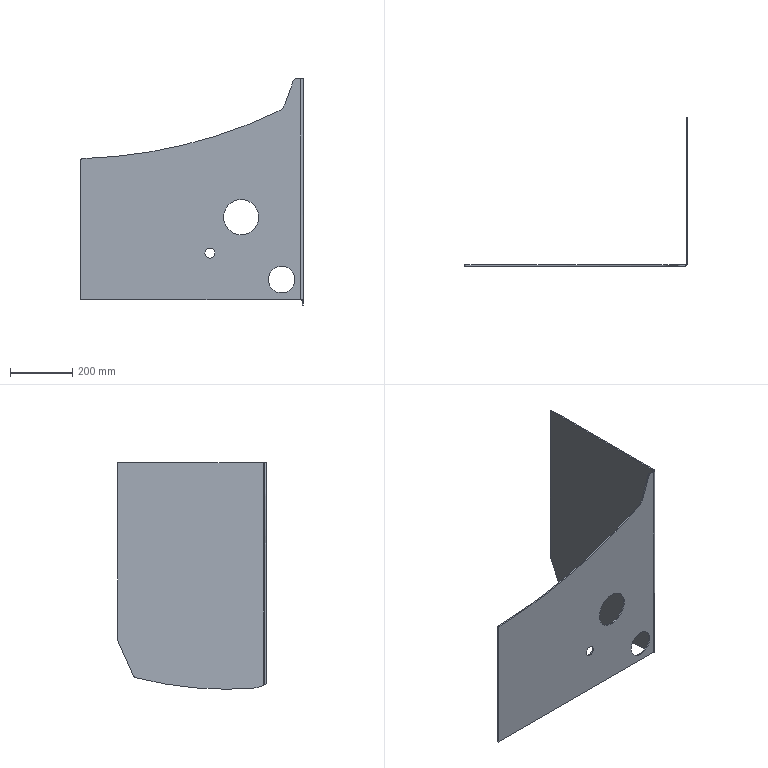Part | SolidWorks | features ICE 3, Fillet 2, FlatPattern 1, SMBaseFlange 1, SheetMetal 1 | 1 solid | 29 faces | box 715 x 476 x 726.29 mm | volume 2754090 mm3 | cylinder 15 | plane 13 | spline 1 | commonest cylinder face diameters 16 x3 20 x2 32.5 x2 85.5 x2 113 x2 12 x1
STEP:
#1=CARTESIAN_POINT('',(-283.75,-476.,-194.));
#2=VERTEX_POINT('',#1);
#3=CARTESIAN_POINT('',(-316.25,-476.,-194.));
#4=VERTEX_POINT('',#3);
#5=CARTESIAN_POINT('',(-300.,-476.,-194.));
#6=DIRECTION('',(0.,1.,0.));
#7=DIRECTION('',(1.,0.,0.));
#8=AXIS2_PLACEMENT_3D('',#5,#6,#7);
#9=CIRCLE('',#8,16.25);
#10=EDGE_CURVE('',#2,#4,#9,.T.);
#11=ORIENTED_EDGE('',*,*,#10,.F.);
#12=CARTESIAN_POINT('',(-283.75,-472.,-194.));
#13=VERTEX_POINT('',#12);
#14=CARTESIAN_POINT('',(-283.75,-476.001,-194.));
#15=DIRECTION('',(0.,1.,0.));
#16=VECTOR('',#15,1000.);
#17=LINE('',#14,#16);
#18=EDGE_CURVE('',#2,#13,#17,.T.);
#19=ORIENTED_EDGE('',*,*,#18,.T.);
#20=CARTESIAN_POINT('',(-316.25,-472.,-194.));
#21=VERTEX_POINT('',#20);
#22=CARTESIAN_POINT('',(-300.,-472.,-194.));
#23=DIRECTION('',(0.,1.,0.));
#24=DIRECTION('',(-1.,0.,0.));
#25=AXIS2_PLACEMENT_3D('',#22,#23,#24);
#26=CIRCLE('',#25,16.25);
#27=EDGE_CURVE('',#13,#21,#26,.T.);
#28=ORIENTED_EDGE('',*,*,#27,.T.);
#29=CARTESIAN_POINT('',(-316.25,-476.001,-194.));
#30=DIRECTION('',(0.,1.,0.));
#31=VECTOR('',#30,1000.);
#32=LINE('',#29,#31);
#33=EDGE_CURVE('',#4,#21,#32,.T.);
#34=ORIENTED_EDGE('',*,*,#33,.F.);
#35=EDGE_LOOP('',(#11,#19,#28,#34));
#36=FACE_OUTER_BOUND('',#35,.T.);
#37=CARTESIAN_POINT('',(-300.,-476.001,-194.));
#38=DIRECTION('',(0.,1.,0.));
#39=DIRECTION('',(-1.,0.,0.));
#40=AXIS2_PLACEMENT_3D('',#37,#38,#39);
#41=CYLINDRICAL_SURFACE('',#40,16.25);
#42=ADVANCED_FACE('',(#36),#41,.F.);
#43=CARTESIAN_POINT('',(-143.5,-476.,-79.));
#44=VERTEX_POINT('',#43);
#45=CARTESIAN_POINT('',(-256.5,-476.,-79.));
#46=VERTEX_POINT('',#45);
#47=CARTESIAN_POINT('',(-200.,-476.,-79.));
#48=DIRECTION('',(0.,1.,0.));
#49=DIRECTION('',(1.,0.,0.));
#50=AXIS2_PLACEMENT_3D('',#47,#48,#49);
#51=CIRCLE('',#50,56.5);
#52=EDGE_CURVE('',#44,#46,#51,.T.);
#53=ORIENTED_EDGE('',*,*,#52,.F.);
#54=CARTESIAN_POINT('',(-143.5,-472.,-79.));
#55=VERTEX_POINT('',#54);
#56=CARTESIAN_POINT('',(-143.5,-476.001,-79.));
#57=DIRECTION('',(0.,1.,0.));
#58=VECTOR('',#57,1000.);
#59=LINE('',#56,#58);
#60=EDGE_CURVE('',#44,#55,#59,.T.);
#61=ORIENTED_EDGE('',*,*,#60,.T.);
#62=CARTESIAN_POINT('',(-256.5,-472.,-79.));
#63=VERTEX_POINT('',#62);
#64=CARTESIAN_POINT('',(-200.,-472.,-79.));
#65=DIRECTION('',(0.,1.,0.));
#66=DIRECTION('',(-1.,0.,0.));
#67=AXIS2_PLACEMENT_3D('',#64,#65,#66);
#68=CIRCLE('',#67,56.5);
#69=EDGE_CURVE('',#55,#63,#68,.T.);
#70=ORIENTED_EDGE('',*,*,#69,.T.);
#71=CARTESIAN_POINT('',(-256.5,-476.001,-79.));
#72=DIRECTION('',(0.,1.,0.));
#73=VECTOR('',#72,1000.);
#74=LINE('',#71,#73);
#75=EDGE_CURVE('',#46,#63,#74,.T.);
#76=ORIENTED_EDGE('',*,*,#75,.F.);
#77=EDGE_LOOP('',(#53,#61,#70,#76));
#78=FACE_OUTER_BOUND('',#77,.T.);
#79=CARTESIAN_POINT('',(-200.,-476.001,-79.));
#80=DIRECTION('',(0.,1.,0.));
#81=DIRECTION('',(-1.,0.,0.));
#82=AXIS2_PLACEMENT_3D('',#79,#80,#81);
#83=CYLINDRICAL_SURFACE('',#82,56.5);
#84=ADVANCED_FACE('',(#78),#83,.F.);
#85=CARTESIAN_POINT('',(-27.25,-476.,-279.));
#86=VERTEX_POINT('',#85);
#87=CARTESIAN_POINT('',(-112.75,-476.,-279.));
#88=VERTEX_POINT('',#87);
#89=CARTESIAN_POINT('',(-70.,-476.,-279.));
#90=DIRECTION('',(0.,1.,0.));
#91=DIRECTION('',(1.,0.,0.));
#92=AXIS2_PLACEMENT_3D('',#89,#90,#91);
#93=CIRCLE('',#92,42.75);
#94=EDGE_CURVE('',#86,#88,#93,.T.);
#95=ORIENTED_EDGE('',*,*,#94,.F.);
#96=CARTESIAN_POINT('',(-27.25,-472.,-279.));
#97=VERTEX_POINT('',#96);
#98=CARTESIAN_POINT('',(-27.25,-476.001,-279.));
#99=DIRECTION('',(0.,1.,0.));
#100=VECTOR('',#99,1000.);
#101=LINE('',#98,#100);
#102=EDGE_CURVE('',#86,#97,#101,.T.);
#103=ORIENTED_EDGE('',*,*,#102,.T.);
#104=CARTESIAN_POINT('',(-112.75,-472.,-279.));
#105=VERTEX_POINT('',#104);
#106=CARTESIAN_POINT('',(-70.,-472.,-279.));
#107=DIRECTION('',(0.,1.,0.));
#108=DIRECTION('',(-1.,0.,0.));
#109=AXIS2_PLACEMENT_3D('',#106,#107,#108);
#110=CIRCLE('',#109,42.75);
#111=EDGE_CURVE('',#97,#105,#110,.T.);
#112=ORIENTED_EDGE('',*,*,#111,.T.);
#113=CARTESIAN_POINT('',(-112.75,-476.001,-279.));
#114=DIRECTION('',(0.,1.,0.));
#115=VECTOR('',#114,1000.);
#116=LINE('',#113,#115);
#117=EDGE_CURVE('',#88,#105,#116,.T.);
#118=ORIENTED_EDGE('',*,*,#117,.F.);
#119=EDGE_LOOP('',(#95,#103,#112,#118));
#120=FACE_OUTER_BOUND('',#119,.T.);
#121=CARTESIAN_POINT('',(-70.,-476.001,-279.));
#122=DIRECTION('',(0.,1.,0.));
#123=DIRECTION('',(-1.,0.,0.));
#124=AXIS2_PLACEMENT_3D('',#121,#122,#123);
#125=CYLINDRICAL_SURFACE('',#124,42.75);
#126=ADVANCED_FACE('',(#120),#125,.F.);
#127=CARTESIAN_POINT('',(-715.,-476.,101.209));
#128=VERTEX_POINT('',#127);
#129=CARTESIAN_POINT('',(-715.,-476.,-343.5));
#130=VERTEX_POINT('',#129);
#131=CARTESIAN_POINT('',(-715.,-476.,365.));
#132=DIRECTION('',(0.,0.,-1.));
#133=VECTOR('',#132,1000.);
#134=LINE('',#131,#133);
#135=EDGE_CURVE('',#128,#130,#134,.T.);
#136=ORIENTED_EDGE('',*,*,#135,.F.);
#137=CARTESIAN_POINT('',(-715.,-472.,101.209));
#138=VERTEX_POINT('',#137);
#139=CARTESIAN_POINT('',(-715.,-476.,101.209));
#140=DIRECTION('',(0.,1.,0.));
#141=VECTOR('',#140,1000.);
#142=LINE('',#139,#141);
#143=EDGE_CURVE('',#128,#138,#142,.T.);
#144=ORIENTED_EDGE('',*,*,#143,.T.);
#145=CARTESIAN_POINT('',(-715.,-472.,-343.5));
#146=VERTEX_POINT('',#145);
#147=CARTESIAN_POINT('',(-715.,-472.,365.));
#148=DIRECTION('',(0.,0.,-1.));
#149=VECTOR('',#148,1000.);
#150=LINE('',#147,#149);
#151=EDGE_CURVE('',#138,#146,#150,.T.);
#152=ORIENTED_EDGE('',*,*,#151,.T.);
#153=CARTESIAN_POINT('',(-715.,-476.,-343.5));
#154=DIRECTION('',(0.,1.,0.));
#155=VECTOR('',#154,1000.);
#156=LINE('',#153,#155);
#157=EDGE_CURVE('',#130,#146,#156,.T.);
#158=ORIENTED_EDGE('',*,*,#157,.F.);
#159=EDGE_LOOP('',(#136,#144,#152,#158));
#160=FACE_OUTER_BOUND('',#159,.T.);
#161=CARTESIAN_POINT('',(-715.,-476.,365.));
#162=DIRECTION('',(-1.,0.,0.));
#163=DIRECTION('',(0.,0.,1.));
#164=AXIS2_PLACEMENT_3D('',#161,#162,#163);
#165=PLANE('',#164);
#166=ADVANCED_FACE('',(#160),#165,.T.);
#167=CARTESIAN_POINT('',(-300.,-472.,-194.));
#168=DIRECTION('',(0.,1.,0.));
#169=DIRECTION('',(-1.,0.,0.));
#170=AXIS2_PLACEMENT_3D('',#167,#168,#169);
#171=CIRCLE('',#170,16.25);
#172=EDGE_CURVE('',#21,#13,#171,.T.);
#173=ORIENTED_EDGE('',*,*,#172,.F.);
#174=ORIENTED_EDGE('',*,*,#27,.F.);
#175=EDGE_LOOP('',(#173,#174));
#176=FACE_BOUND('',#175,.T.);
#177=CARTESIAN_POINT('',(-200.,-472.,-79.));
#178=DIRECTION('',(0.,1.,0.));
#179=DIRECTION('',(-1.,0.,0.));
#180=AXIS2_PLACEMENT_3D('',#177,#178,#179);
#181=CIRCLE('',#180,56.5);
#182=EDGE_CURVE('',#63,#55,#181,.T.);
#183=ORIENTED_EDGE('',*,*,#182,.F.);
#184=ORIENTED_EDGE('',*,*,#69,.F.);
#185=EDGE_LOOP('',(#183,#184));
#186=FACE_BOUND('',#185,.T.);
#187=CARTESIAN_POINT('',(-70.,-472.,-279.));
#188=DIRECTION('',(0.,1.,0.));
#189=DIRECTION('',(-1.,0.,0.));
#190=AXIS2_PLACEMENT_3D('',#187,#188,#189);
#191=CIRCLE('',#190,42.75);
#192=EDGE_CURVE('',#105,#97,#191,.T.);
#193=ORIENTED_EDGE('',*,*,#192,.F.);
#194=ORIENTED_EDGE('',*,*,#111,.F.);
#195=EDGE_LOOP('',(#193,#194));
#196=FACE_BOUND('',#195,.T.);
#197=ORIENTED_EDGE('',*,*,#151,.F.);
#198=CARTESIAN_POINT('',(-707.231,-472.,109.205));
#199=VERTEX_POINT('',#198);
#200=CARTESIAN_POINT('',(-707.,-472.,101.209));
#201=DIRECTION('',(0.,1.,0.));
#202=DIRECTION('',(1.,0.,0.));
#203=AXIS2_PLACEMENT_3D('',#200,#201,#202);
#204=CIRCLE('',#203,8.);
#205=EDGE_CURVE('',#138,#199,#204,.T.);
#206=ORIENTED_EDGE('',*,*,#205,.T.);
#207=CARTESIAN_POINT('',(-82.003,-472.,259.931));
#208=VERTEX_POINT('',#207);
#209=CARTESIAN_POINT('',(-752.366,-472.,1668.552));
#210=DIRECTION('',(0.,1.,0.));
#211=DIRECTION('',(1.,0.,0.));
#212=AXIS2_PLACEMENT_3D('',#209,#210,#211);
#213=CIRCLE('',#212,1560.);
#214=EDGE_CURVE('',#208,#199,#213,.T.);
#215=ORIENTED_EDGE('',*,*,#214,.F.);
#216=CARTESIAN_POINT('',(-59.054,-472.,285.174));
#217=VERTEX_POINT('',#216);
#218=CARTESIAN_POINT('',(-101.341,-472.,300.565));
#219=DIRECTION('',(0.,1.,0.));
#220=DIRECTION('',(1.,0.,0.));
#221=AXIS2_PLACEMENT_3D('',#218,#219,#220);
#222=CIRCLE('',#221,45.);
#223=EDGE_CURVE('',#217,#208,#222,.T.);
#224=ORIENTED_EDGE('',*,*,#223,.F.);
#225=CARTESIAN_POINT('',(-32.395,-472.,358.42));
#226=VERTEX_POINT('',#225);
#227=CARTESIAN_POINT('',(-30.,-472.,365.));
#228=DIRECTION('',(-0.342,0.,-0.9397));
#229=VECTOR('',#228,1000.);
#230=LINE('',#227,#229);
#231=EDGE_CURVE('',#226,#217,#230,.T.);
#232=ORIENTED_EDGE('',*,*,#231,.F.);
#233=CARTESIAN_POINT('',(-22.998,-472.,365.));
#234=VERTEX_POINT('',#233);
#235=CARTESIAN_POINT('',(-22.998,-472.,355.));
#236=DIRECTION('',(0.,1.,0.));
#237=DIRECTION('',(1.,0.,0.));
#238=AXIS2_PLACEMENT_3D('',#235,#236,#237);
#239=CIRCLE('',#238,10.);
#240=EDGE_CURVE('',#226,#234,#239,.T.);
#241=ORIENTED_EDGE('',*,*,#240,.T.);
#242=CARTESIAN_POINT('',(-10.,-472.,365.));
#243=VERTEX_POINT('',#242);
#244=CARTESIAN_POINT('',(0.,-472.,365.));
#245=DIRECTION('',(-1.,0.,0.));
#246=VECTOR('',#245,1000.);
#247=LINE('',#244,#246);
#248=EDGE_CURVE('',#243,#234,#247,.T.);
#249=ORIENTED_EDGE('',*,*,#248,.F.);
#250=CARTESIAN_POINT('',(-10.,-472.,-343.5));
#251=VERTEX_POINT('',#250);
#252=CARTESIAN_POINT('',(-10.,-472.,365.));
#253=DIRECTION('',(0.,0.,-1.));
#254=VECTOR('',#253,1000.);
#255=LINE('',#252,#254);
#256=EDGE_CURVE('',#243,#251,#255,.T.);
#257=ORIENTED_EDGE('',*,*,#256,.T.);
#258=CARTESIAN_POINT('',(0.,-472.,-343.5));
#259=DIRECTION('',(-1.,0.,0.));
#260=VECTOR('',#259,1000.);
#261=LINE('',#258,#260);
#262=EDGE_CURVE('',#251,#146,#261,.T.);
#263=ORIENTED_EDGE('',*,*,#262,.T.);
#264=EDGE_LOOP('',(#197,#206,#215,#224,#232,#241,#249,#257,#263));
#265=FACE_OUTER_BOUND('',#264,.T.);
#266=CARTESIAN_POINT('',(0.,-472.,365.));
#267=DIRECTION('',(0.,-1.,0.));
#268=DIRECTION('',(1.,0.,0.));
#269=AXIS2_PLACEMENT_3D('',#266,#267,#268);
#270=PLANE('',#269);
#271=ADVANCED_FACE('',(#176,#186,#196,#265),#270,.F.);
#272=CARTESIAN_POINT('',(-300.,-476.,-194.));
#273=DIRECTION('',(0.,1.,0.));
#274=DIRECTION('',(1.,0.,0.));
#275=AXIS2_PLACEMENT_3D('',#272,#273,#274);
#276=CIRCLE('',#275,16.25);
#277=EDGE_CURVE('',#4,#2,#276,.T.);
#278=ORIENTED_EDGE('',*,*,#277,.T.);
#279=ORIENTED_EDGE('',*,*,#10,.T.);
#280=EDGE_LOOP('',(#278,#279));
#281=FACE_BOUND('',#280,.T.);
#282=CARTESIAN_POINT('',(-200.,-476.,-79.));
#283=DIRECTION('',(0.,1.,0.));
#284=DIRECTION('',(1.,0.,0.));
#285=AXIS2_PLACEMENT_3D('',#282,#283,#284);
#286=CIRCLE('',#285,56.5);
#287=EDGE_CURVE('',#46,#44,#286,.T.);
#288=ORIENTED_EDGE('',*,*,#287,.T.);
#289=ORIENTED_EDGE('',*,*,#52,.T.);
#290=EDGE_LOOP('',(#288,#289));
#291=FACE_BOUND('',#290,.T.);
#292=CARTESIAN_POINT('',(-70.,-476.,-279.));
#293=DIRECTION('',(0.,1.,0.));
#294=DIRECTION('',(1.,0.,0.));
#295=AXIS2_PLACEMENT_3D('',#292,#293,#294);
#296=CIRCLE('',#295,42.75);
#297=EDGE_CURVE('',#88,#86,#296,.T.);
#298=ORIENTED_EDGE('',*,*,#297,.T.);
#299=ORIENTED_EDGE('',*,*,#94,.T.);
#300=EDGE_LOOP('',(#298,#299));
#301=FACE_BOUND('',#300,.T.);
#302=CARTESIAN_POINT('',(-82.003,-476.,259.931));
#303=VERTEX_POINT('',#302);
#304=CARTESIAN_POINT('',(-707.231,-476.,109.205));
#305=VERTEX_POINT('',#304);
#306=CARTESIAN_POINT('',(-752.366,-476.,1668.552));
#307=DIRECTION('',(0.,1.,0.));
#308=DIRECTION('',(1.,0.,0.));
#309=AXIS2_PLACEMENT_3D('',#306,#307,#308);
#310=CIRCLE('',#309,1560.);
#311=EDGE_CURVE('',#303,#305,#310,.T.);
#312=ORIENTED_EDGE('',*,*,#311,.T.);
#313=CARTESIAN_POINT('',(-707.,-476.,101.209));
#314=DIRECTION('',(0.,-1.,0.));
#315=DIRECTION('',(1.,0.,0.));
#316=AXIS2_PLACEMENT_3D('',#313,#314,#315);
#317=CIRCLE('',#316,8.);
#318=EDGE_CURVE('',#305,#128,#317,.T.);
#319=ORIENTED_EDGE('',*,*,#318,.T.);
#320=ORIENTED_EDGE('',*,*,#135,.T.);
#321=CARTESIAN_POINT('',(-10.,-476.,-343.5));
#322=VERTEX_POINT('',#321);
#323=CARTESIAN_POINT('',(0.,-476.,-343.5));
#324=DIRECTION('',(-1.,0.,0.));
#325=VECTOR('',#324,1000.);
#326=LINE('',#323,#325);
#327=EDGE_CURVE('',#322,#130,#326,.T.);
#328=ORIENTED_EDGE('',*,*,#327,.F.);
#329=CARTESIAN_POINT('',(-10.,-476.,365.));
#330=VERTEX_POINT('',#329);
#331=CARTESIAN_POINT('',(-10.,-476.,365.));
#332=DIRECTION('',(0.,0.,-1.));
#333=VECTOR('',#332,1000.);
#334=LINE('',#331,#333);
#335=EDGE_CURVE('',#330,#322,#334,.T.);
#336=ORIENTED_EDGE('',*,*,#335,.F.);
#337=CARTESIAN_POINT('',(-22.998,-476.,365.));
#338=VERTEX_POINT('',#337);
#339=CARTESIAN_POINT('',(0.,-476.,365.));
#340=DIRECTION('',(-1.,0.,0.));
#341=VECTOR('',#340,1000.);
#342=LINE('',#339,#341);
#343=EDGE_CURVE('',#330,#338,#342,.T.);
#344=ORIENTED_EDGE('',*,*,#343,.T.);
#345=CARTESIAN_POINT('',(-32.395,-476.,358.42));
#346=VERTEX_POINT('',#345);
#347=CARTESIAN_POINT('',(-22.998,-476.,355.));
#348=DIRECTION('',(0.,-1.,0.));
#349=DIRECTION('',(1.,0.,0.));
#350=AXIS2_PLACEMENT_3D('',#347,#348,#349);
#351=CIRCLE('',#350,10.);
#352=EDGE_CURVE('',#338,#346,#351,.T.);
#353=ORIENTED_EDGE('',*,*,#352,.T.);
#354=CARTESIAN_POINT('',(-59.054,-476.,285.174));
#355=VERTEX_POINT('',#354);
#356=CARTESIAN_POINT('',(-30.,-476.,365.));
#357=DIRECTION('',(-0.342,0.,-0.9397));
#358=VECTOR('',#357,1000.);
#359=LINE('',#356,#358);
#360=EDGE_CURVE('',#346,#355,#359,.T.);
#361=ORIENTED_EDGE('',*,*,#360,.T.);
#362=CARTESIAN_POINT('',(-101.341,-476.,300.565));
#363=DIRECTION('',(0.,1.,0.));
#364=DIRECTION('',(1.,0.,0.));
#365=AXIS2_PLACEMENT_3D('',#362,#363,#364);
#366=CIRCLE('',#365,45.);
#367=EDGE_CURVE('',#355,#303,#366,.T.);
#368=ORIENTED_EDGE('',*,*,#367,.T.);
#369=EDGE_LOOP('',(#312,#319,#320,#328,#336,#344,#353,#361,#368));
#370=FACE_OUTER_BOUND('',#369,.T.);
#371=CARTESIAN_POINT('',(0.,-476.,365.));
#372=DIRECTION('',(0.,-1.,0.));
#373=DIRECTION('',(1.,0.,0.));
#374=AXIS2_PLACEMENT_3D('',#371,#372,#373);
#375=PLANE('',#374);
#376=ADVANCED_FACE('',(#281,#291,#301,#370),#375,.T.);
#377=ORIENTED_EDGE('',*,*,#335,.T.);
#378=CARTESIAN_POINT('',(0.,-466.,-348.076));
#379=VERTEX_POINT('',#378);
#380=CARTESIAN_POINT('',(0.,-466.,-348.076));
#381=CARTESIAN_POINT('',(0.,-471.858,-345.396));
#382=CARTESIAN_POINT('',(-4.142,-476.,-343.5));
#383=CARTESIAN_POINT('',(-10.,-476.,-343.5));
#384=(BOUNDED_CURVE()B_SPLINE_CURVE(3,(#380,#381,#382,#383),.UNSPECIFIED.,.F.,.F.)B_SPLINE_CURVE_WITH_KNOTS((4,4),(1.571,3.142),.UNSPECIFIED.)CURVE()GEOMETRIC_REPRESENTATION_ITEM()RATIONAL_B_SPLINE_CURVE((1.,0.8047,0.8047,1.))REPRESENTATION_ITEM(''));
#385=EDGE_CURVE('',#379,#322,#384,.T.);
#386=ORIENTED_EDGE('',*,*,#385,.F.);
#387=CARTESIAN_POINT('',(0.,-466.,365.));
#388=VERTEX_POINT('',#387);
#389=CARTESIAN_POINT('',(0.,-466.,365.));
#390=DIRECTION('',(0.,0.,-1.));
#391=VECTOR('',#390,1000.);
#392=LINE('',#389,#391);
#393=EDGE_CURVE('',#388,#379,#392,.T.);
#394=ORIENTED_EDGE('',*,*,#393,.F.);
#395=CARTESIAN_POINT('',(-10.,-466.,365.));
#396=DIRECTION('',(0.,0.,-1.));
#397=DIRECTION('',(1.,0.,0.));
#398=AXIS2_PLACEMENT_3D('',#395,#396,#397);
#399=CIRCLE('',#398,10.);
#400=EDGE_CURVE('',#388,#330,#399,.T.);
#401=ORIENTED_EDGE('',*,*,#400,.T.);
#402=EDGE_LOOP('',(#377,#386,#394,#401));
#403=FACE_OUTER_BOUND('',#402,.T.);
#404=CARTESIAN_POINT('',(-10.,-466.,365.));
#405=DIRECTION('',(0.,0.,-1.));
#406=DIRECTION('',(-1.,0.,0.));
#407=AXIS2_PLACEMENT_3D('',#404,#405,#406);
#408=CYLINDRICAL_SURFACE('',#407,10.);
#409=ADVANCED_FACE('',(#403),#408,.T.);
#410=CARTESIAN_POINT('',(0.,-0.7029,-207.064));
#411=VERTEX_POINT('',#410);
#412=CARTESIAN_POINT('',(0.,-51.233,-319.513));
#413=VERTEX_POINT('',#412);
#414=CARTESIAN_POINT('',(0.,213.292,269.155));
#415=DIRECTION('',(0.,-0.4099,-0.9121));
#416=VECTOR('',#415,1000.);
#417=LINE('',#414,#416);
#418=EDGE_CURVE('',#411,#413,#417,.T.);
#419=ORIENTED_EDGE('',*,*,#418,.F.);
#420=CARTESIAN_POINT('',(0.,0.,-203.785));
#421=VERTEX_POINT('',#420);
#422=CARTESIAN_POINT('',(0.,-8.,-203.785));
#423=DIRECTION('',(1.,0.,0.));
#424=DIRECTION('',(0.,1.,0.));
#425=AXIS2_PLACEMENT_3D('',#422,#423,#424);
#426=CIRCLE('',#425,8.);
#427=EDGE_CURVE('',#411,#421,#426,.T.);
#428=ORIENTED_EDGE('',*,*,#427,.T.);
#429=CARTESIAN_POINT('',(0.,0.,365.));
#430=VERTEX_POINT('',#429);
#431=CARTESIAN_POINT('',(0.,0.,365.));
#432=DIRECTION('',(0.,0.,-1.));
#433=VECTOR('',#432,1000.);
#434=LINE('',#431,#433);
#435=EDGE_CURVE('',#430,#421,#434,.T.);
#436=ORIENTED_EDGE('',*,*,#435,.F.);
#437=CARTESIAN_POINT('',(0.,0.,365.));
#438=DIRECTION('',(0.,-1.,0.));
#439=VECTOR('',#438,1000.);
#440=LINE('',#437,#439);
#441=EDGE_CURVE('',#430,#388,#440,.T.);
#442=ORIENTED_EDGE('',*,*,#441,.T.);
#443=ORIENTED_EDGE('',*,*,#393,.T.);
#444=CARTESIAN_POINT('',(0.,-446.5,-357.));
#445=VERTEX_POINT('',#444);
#446=CARTESIAN_POINT('',(0.,-350.509,-400.928));
#447=DIRECTION('',(0.,-0.9093,0.4161));
#448=VECTOR('',#447,1000.);
#449=LINE('',#446,#448);
#450=EDGE_CURVE('',#445,#379,#449,.T.);
#451=ORIENTED_EDGE('',*,*,#450,.F.);
#452=CARTESIAN_POINT('',(0.,-56.51,-323.975));
#453=VERTEX_POINT('',#452);
#454=CARTESIAN_POINT('',(0.,-347.212,789.71));
#455=DIRECTION('',(-1.,0.,0.));
#456=DIRECTION('',(0.,1.,0.));
#457=AXIS2_PLACEMENT_3D('',#454,#455,#456);
#458=CIRCLE('',#457,1151.);
#459=EDGE_CURVE('',#453,#445,#458,.T.);
#460=ORIENTED_EDGE('',*,*,#459,.F.);
#461=CARTESIAN_POINT('',(0.,-58.53,-316.234));
#462=DIRECTION('',(1.,0.,0.));
#463=DIRECTION('',(0.,1.,0.));
#464=AXIS2_PLACEMENT_3D('',#461,#462,#463);
#465=CIRCLE('',#464,8.);
#466=EDGE_CURVE('',#453,#413,#465,.T.);
#467=ORIENTED_EDGE('',*,*,#466,.T.);
#468=EDGE_LOOP('',(#419,#428,#436,#442,#443,#451,#460,#467));
#469=FACE_OUTER_BOUND('',#468,.T.);
#470=CARTESIAN_POINT('',(0.,0.,365.));
#471=DIRECTION('',(1.,0.,0.));
#472=DIRECTION('',(0.,1.,0.));
#473=AXIS2_PLACEMENT_3D('',#470,#471,#472);
#474=PLANE('',#473);
#475=ADVANCED_FACE('',(#469),#474,.T.);
#476=ORIENTED_EDGE('',*,*,#435,.T.);
#477=CARTESIAN_POINT('',(-4.,0.,-203.785));
#478=VERTEX_POINT('',#477);
#479=CARTESIAN_POINT('',(-4.,0.,-203.785));
#480=DIRECTION('',(-1.,0.,0.));
#481=VECTOR('',#480,1000.);
#482=LINE('',#479,#481);
#483=EDGE_CURVE('',#421,#478,#482,.T.);
#484=ORIENTED_EDGE('',*,*,#483,.T.);
#485=CARTESIAN_POINT('',(-4.,0.,365.));
#486=VERTEX_POINT('',#485);
#487=CARTESIAN_POINT('',(-4.,0.,365.));
#488=DIRECTION('',(0.,0.,-1.));
#489=VECTOR('',#488,1000.);
#490=LINE('',#487,#489);
#491=EDGE_CURVE('',#486,#478,#490,.T.);
#492=ORIENTED_EDGE('',*,*,#491,.F.);
#493=CARTESIAN_POINT('',(-4.,0.,365.));
#494=DIRECTION('',(1.,0.,0.));
#495=VECTOR('',#494,1000.);
#496=LINE('',#493,#495);
#497=EDGE_CURVE('',#486,#430,#496,.T.);
#498=ORIENTED_EDGE('',*,*,#497,.T.);
#499=EDGE_LOOP('',(#476,#484,#492,#498));
#500=FACE_OUTER_BOUND('',#499,.T.);
#501=CARTESIAN_POINT('',(-4.,0.,365.));
#502=DIRECTION('',(0.,1.,0.));
#503=DIRECTION('',(-1.,0.,0.));
#504=AXIS2_PLACEMENT_3D('',#501,#502,#503);
#505=PLANE('',#504);
#506=ADVANCED_FACE('',(#500),#505,.T.);
#507=ORIENTED_EDGE('',*,*,#491,.T.);
#508=CARTESIAN_POINT('',(-4.,-0.7029,-207.064));
#509=VERTEX_POINT('',#508);
#510=CARTESIAN_POINT('',(-4.,-8.,-203.785));
#511=DIRECTION('',(-1.,0.,0.));
#512=DIRECTION('',(0.,1.,0.));
#513=AXIS2_PLACEMENT_3D('',#510,#511,#512);
#514=CIRCLE('',#513,8.);
#515=EDGE_CURVE('',#478,#509,#514,.T.);
#516=ORIENTED_EDGE('',*,*,#515,.T.);
#517=CARTESIAN_POINT('',(-4.,-51.233,-319.513));
#518=VERTEX_POINT('',#517);
#519=CARTESIAN_POINT('',(-4.,213.292,269.155));
#520=DIRECTION('',(0.,-0.4099,-0.9121));
#521=VECTOR('',#520,1000.);
#522=LINE('',#519,#521);
#523=EDGE_CURVE('',#509,#518,#522,.T.);
#524=ORIENTED_EDGE('',*,*,#523,.T.);
#525=CARTESIAN_POINT('',(-4.,-56.51,-323.975));
#526=VERTEX_POINT('',#525);
#527=CARTESIAN_POINT('',(-4.,-58.53,-316.234));
#528=DIRECTION('',(-1.,0.,0.));
#529=DIRECTION('',(0.,1.,0.));
#530=AXIS2_PLACEMENT_3D('',#527,#528,#529);
#531=CIRCLE('',#530,8.);
#532=EDGE_CURVE('',#518,#526,#531,.T.);
#533=ORIENTED_EDGE('',*,*,#532,.T.);
#534=CARTESIAN_POINT('',(-4.,-446.5,-357.));
#535=VERTEX_POINT('',#534);
#536=CARTESIAN_POINT('',(-4.,-347.212,789.71));
#537=DIRECTION('',(-1.,0.,0.));
#538=DIRECTION('',(0.,1.,0.));
#539=AXIS2_PLACEMENT_3D('',#536,#537,#538);
#540=CIRCLE('',#539,1151.);
#541=EDGE_CURVE('',#526,#535,#540,.T.);
#542=ORIENTED_EDGE('',*,*,#541,.T.);
#543=CARTESIAN_POINT('',(-4.,-466.,-348.076));
#544=VERTEX_POINT('',#543);
#545=CARTESIAN_POINT('',(-4.,-350.509,-400.928));
#546=DIRECTION('',(0.,-0.9093,0.4161));
#547=VECTOR('',#546,1000.);
#548=LINE('',#545,#547);
#549=EDGE_CURVE('',#535,#544,#548,.T.);
#550=ORIENTED_EDGE('',*,*,#549,.T.);
#551=CARTESIAN_POINT('',(-4.,-466.,365.));
#552=VERTEX_POINT('',#551);
#553=CARTESIAN_POINT('',(-4.,-466.,365.));
#554=DIRECTION('',(0.,0.,-1.));
#555=VECTOR('',#554,1000.);
#556=LINE('',#553,#555);
#557=EDGE_CURVE('',#552,#544,#556,.T.);
#558=ORIENTED_EDGE('',*,*,#557,.F.);
#559=CARTESIAN_POINT('',(-4.,0.,365.));
#560=DIRECTION('',(0.,-1.,0.));
#561=VECTOR('',#560,1000.);
#562=LINE('',#559,#561);
#563=EDGE_CURVE('',#486,#552,#562,.T.);
#564=ORIENTED_EDGE('',*,*,#563,.F.);
#565=EDGE_LOOP('',(#507,#516,#524,#533,#542,#550,#558,#564));
#566=FACE_OUTER_BOUND('',#565,.T.);
#567=CARTESIAN_POINT('',(-4.,0.,365.));
#568=DIRECTION('',(1.,0.,0.));
#569=DIRECTION('',(0.,1.,0.));
#570=AXIS2_PLACEMENT_3D('',#567,#568,#569);
#571=PLANE('',#570);
#572=ADVANCED_FACE('',(#566),#571,.F.);
#573=CARTESIAN_POINT('',(-4.,-466.,-348.076));
#574=CARTESIAN_POINT('',(-4.,-469.515,-345.396));
#575=CARTESIAN_POINT('',(-6.485,-472.,-343.5));
#576=CARTESIAN_POINT('',(-10.,-472.,-343.5));
#577=(BOUNDED_CURVE()B_SPLINE_CURVE(3,(#573,#574,#575,#576),.UNSPECIFIED.,.F.,.F.)B_SPLINE_CURVE_WITH_KNOTS((4,4),(1.571,3.142),.UNSPECIFIED.)CURVE()GEOMETRIC_REPRESENTATION_ITEM()RATIONAL_B_SPLINE_CURVE((1.,0.8047,0.8047,1.))REPRESENTATION_ITEM(''));
#578=EDGE_CURVE('',#544,#251,#577,.T.);
#579=ORIENTED_EDGE('',*,*,#578,.T.);
#580=ORIENTED_EDGE('',*,*,#256,.F.);
#581=CARTESIAN_POINT('',(-10.,-466.,365.));
#582=DIRECTION('',(0.,0.,-1.));
#583=DIRECTION('',(1.,0.,0.));
#584=AXIS2_PLACEMENT_3D('',#581,#582,#583);
#585=CIRCLE('',#584,6.);
#586=EDGE_CURVE('',#552,#243,#585,.T.);
#587=ORIENTED_EDGE('',*,*,#586,.F.);
#588=ORIENTED_EDGE('',*,*,#557,.T.);
#589=EDGE_LOOP('',(#579,#580,#587,#588));
#590=FACE_OUTER_BOUND('',#589,.T.);
#591=CARTESIAN_POINT('',(-10.,-466.,365.));
#592=DIRECTION('',(0.,0.,-1.));
#593=DIRECTION('',(-1.,0.,0.));
#594=AXIS2_PLACEMENT_3D('',#591,#592,#593);
#595=CYLINDRICAL_SURFACE('',#594,6.);
#596=ADVANCED_FACE('',(#590),#595,.F.);
#597=ORIENTED_EDGE('',*,*,#248,.T.);
#598=CARTESIAN_POINT('',(-22.998,-466.,365.));
#599=DIRECTION('',(0.,-1.,0.));
#600=VECTOR('',#599,1000.);
#601=LINE('',#598,#600);
#602=EDGE_CURVE('',#234,#338,#601,.T.);
#603=ORIENTED_EDGE('',*,*,#602,.T.);
#604=ORIENTED_EDGE('',*,*,#343,.F.);
#605=CARTESIAN_POINT('',(-10.,-476.,365.));
#606=DIRECTION('',(0.,1.,0.));
#607=VECTOR('',#606,1000.);
#608=LINE('',#605,#607);
#609=EDGE_CURVE('',#330,#243,#608,.T.);
#610=ORIENTED_EDGE('',*,*,#609,.T.);
#611=EDGE_LOOP('',(#597,#603,#604,#610));
#612=FACE_OUTER_BOUND('',#611,.T.);
#613=CARTESIAN_POINT('',(-4.,-466.,365.));
#614=DIRECTION('',(0.,0.,1.));
#615=DIRECTION('',(1.,0.,0.));
#616=AXIS2_PLACEMENT_3D('',#613,#614,#615);
#617=PLANE('',#616);
#618=ADVANCED_FACE('',(#612),#617,.T.);
#619=ORIENTED_EDGE('',*,*,#609,.F.);
#620=ORIENTED_EDGE('',*,*,#400,.F.);
#621=CARTESIAN_POINT('',(-4.,-466.,365.));
#622=DIRECTION('',(1.,0.,0.));
#623=VECTOR('',#622,1000.);
#624=LINE('',#621,#623);
#625=EDGE_CURVE('',#552,#388,#624,.T.);
#626=ORIENTED_EDGE('',*,*,#625,.F.);
#627=ORIENTED_EDGE('',*,*,#586,.T.);
#628=EDGE_LOOP('',(#619,#620,#626,#627));
#629=FACE_OUTER_BOUND('',#628,.T.);
#630=CARTESIAN_POINT('',(-10.,-476.,365.));
#631=DIRECTION('',(0.,0.,1.));
#632=DIRECTION('',(1.,0.,0.));
#633=AXIS2_PLACEMENT_3D('',#630,#631,#632);
#634=PLANE('',#633);
#635=ADVANCED_FACE('',(#629),#634,.T.);
#636=ORIENTED_EDGE('',*,*,#563,.T.);
#637=ORIENTED_EDGE('',*,*,#625,.T.);
#638=ORIENTED_EDGE('',*,*,#441,.F.);
#639=ORIENTED_EDGE('',*,*,#497,.F.);
#640=EDGE_LOOP('',(#636,#637,#638,#639));
#641=FACE_OUTER_BOUND('',#640,.T.);
#642=CARTESIAN_POINT('',(-10.,-466.,365.));
#643=DIRECTION('',(0.,0.,1.));
#644=DIRECTION('',(1.,0.,0.));
#645=AXIS2_PLACEMENT_3D('',#642,#643,#644);
#646=PLANE('',#645);
#647=ADVANCED_FACE('',(#641),#646,.T.);
#648=CARTESIAN_POINT('',(-82.003,-476.,259.931));
#649=DIRECTION('',(0.,1.,0.));
#650=VECTOR('',#649,1000.);
#651=LINE('',#648,#650);
#652=EDGE_CURVE('',#303,#208,#651,.T.);
#653=ORIENTED_EDGE('',*,*,#652,.F.);
#654=ORIENTED_EDGE('',*,*,#367,.F.);
#655=CARTESIAN_POINT('',(-59.054,-476.,285.174));
#656=DIRECTION('',(0.,1.,0.));
#657=VECTOR('',#656,1000.);
#658=LINE('',#655,#657);
#659=EDGE_CURVE('',#355,#217,#658,.T.);
#660=ORIENTED_EDGE('',*,*,#659,.T.);
#661=ORIENTED_EDGE('',*,*,#223,.T.);
#662=EDGE_LOOP('',(#653,#654,#660,#661));
#663=FACE_OUTER_BOUND('',#662,.T.);
#664=CARTESIAN_POINT('',(-101.341,-476.,300.565));
#665=DIRECTION('',(0.,-1.,0.));
#666=DIRECTION('',(1.,0.,0.));
#667=AXIS2_PLACEMENT_3D('',#664,#665,#666);
#668=CYLINDRICAL_SURFACE('',#667,45.);
#669=ADVANCED_FACE('',(#663),#668,.F.);
#670=ORIENTED_EDGE('',*,*,#360,.F.);
#671=CARTESIAN_POINT('',(-32.395,-476.,358.42));
#672=DIRECTION('',(0.,1.,0.));
#673=VECTOR('',#672,1000.);
#674=LINE('',#671,#673);
#675=EDGE_CURVE('',#346,#226,#674,.T.);
#676=ORIENTED_EDGE('',*,*,#675,.T.);
#677=ORIENTED_EDGE('',*,*,#231,.T.);
#678=ORIENTED_EDGE('',*,*,#659,.F.);
#679=EDGE_LOOP('',(#670,#676,#677,#678));
#680=FACE_OUTER_BOUND('',#679,.T.);
#681=CARTESIAN_POINT('',(-30.,-476.,365.));
#682=DIRECTION('',(-0.9397,0.,0.342));
#683=DIRECTION('',(-0.342,0.,-0.9397));
#684=AXIS2_PLACEMENT_3D('',#681,#682,#683);
#685=PLANE('',#684);
#686=ADVANCED_FACE('',(#680),#685,.T.);
#687=ORIENTED_EDGE('',*,*,#214,.T.);
#688=CARTESIAN_POINT('',(-707.231,-476.,109.205));
#689=DIRECTION('',(0.,-1.,0.));
#690=VECTOR('',#689,1000.);
#691=LINE('',#688,#690);
#692=EDGE_CURVE('',#199,#305,#691,.T.);
#693=ORIENTED_EDGE('',*,*,#692,.T.);
#694=ORIENTED_EDGE('',*,*,#311,.F.);
#695=ORIENTED_EDGE('',*,*,#652,.T.);
#696=EDGE_LOOP('',(#687,#693,#694,#695));
#697=FACE_OUTER_BOUND('',#696,.T.);
#698=CARTESIAN_POINT('',(-752.366,-476.,1668.552));
#699=DIRECTION('',(0.,-1.,0.));
#700=DIRECTION('',(1.,0.,0.));
#701=AXIS2_PLACEMENT_3D('',#698,#699,#700);
#702=CYLINDRICAL_SURFACE('',#701,1560.);
#703=ADVANCED_FACE('',(#697),#702,.F.);
#704=CARTESIAN_POINT('',(-4.,-466.,-348.076));
#705=DIRECTION('',(1.,0.,0.));
#706=VECTOR('',#705,1000.);
#707=LINE('',#704,#706);
#708=EDGE_CURVE('',#544,#379,#707,.T.);
#709=ORIENTED_EDGE('',*,*,#708,.F.);
#710=ORIENTED_EDGE('',*,*,#549,.F.);
#711=CARTESIAN_POINT('',(-4.,-446.5,-357.));
#712=DIRECTION('',(1.,0.,0.));
#713=VECTOR('',#712,1000.);
#714=LINE('',#711,#713);
#715=EDGE_CURVE('',#535,#445,#714,.T.);
#716=ORIENTED_EDGE('',*,*,#715,.T.);
#717=ORIENTED_EDGE('',*,*,#450,.T.);
#718=EDGE_LOOP('',(#709,#710,#716,#717));
#719=FACE_OUTER_BOUND('',#718,.T.);
#720=CARTESIAN_POINT('',(-4.,-350.509,-400.928));
#721=DIRECTION('',(0.,0.4161,0.9093));
#722=DIRECTION('',(0.,-0.9093,0.4161));
#723=AXIS2_PLACEMENT_3D('',#720,#721,#722);
#724=PLANE('',#723);
#725=ADVANCED_FACE('',(#719),#724,.F.);
#726=ORIENTED_EDGE('',*,*,#541,.F.);
#727=CARTESIAN_POINT('',(-4.,-56.51,-323.975));
#728=DIRECTION('',(1.,0.,0.));
#729=VECTOR('',#728,1000.);
#730=LINE('',#727,#729);
#731=EDGE_CURVE('',#526,#453,#730,.T.);
#732=ORIENTED_EDGE('',*,*,#731,.T.);
#733=ORIENTED_EDGE('',*,*,#459,.T.);
#734=ORIENTED_EDGE('',*,*,#715,.F.);
#735=EDGE_LOOP('',(#726,#732,#733,#734));
#736=FACE_OUTER_BOUND('',#735,.T.);
#737=CARTESIAN_POINT('',(-4.,-347.212,789.71));
#738=DIRECTION('',(1.,0.,0.));
#739=DIRECTION('',(0.,1.,0.));
#740=AXIS2_PLACEMENT_3D('',#737,#738,#739);
#741=CYLINDRICAL_SURFACE('',#740,1151.);
#742=ADVANCED_FACE('',(#736),#741,.T.);
#743=ORIENTED_EDGE('',*,*,#523,.F.);
#744=CARTESIAN_POINT('',(-4.,-0.7029,-207.064));
#745=DIRECTION('',(1.,0.,0.));
#746=VECTOR('',#745,1000.);
#747=LINE('',#744,#746);
#748=EDGE_CURVE('',#509,#411,#747,.T.);
#749=ORIENTED_EDGE('',*,*,#748,.T.);
#750=ORIENTED_EDGE('',*,*,#418,.T.);
#751=CARTESIAN_POINT('',(-4.,-51.233,-319.513));
#752=DIRECTION('',(-1.,0.,0.));
#753=VECTOR('',#752,1000.);
#754=LINE('',#751,#753);
#755=EDGE_CURVE('',#413,#518,#754,.T.);
#756=ORIENTED_EDGE('',*,*,#755,.T.);
#757=EDGE_LOOP('',(#743,#749,#750,#756));
#758=FACE_OUTER_BOUND('',#757,.T.);
#759=CARTESIAN_POINT('',(-4.,213.292,269.155));
#760=DIRECTION('',(0.,-0.9121,0.4099));
#761=DIRECTION('',(0.,-0.4099,-0.9121));
#762=AXIS2_PLACEMENT_3D('',#759,#760,#761);
#763=PLANE('',#762);
#764=ADVANCED_FACE('',(#758),#763,.F.);
#765=ORIENTED_EDGE('',*,*,#327,.T.);
#766=ORIENTED_EDGE('',*,*,#157,.T.);
#767=ORIENTED_EDGE('',*,*,#262,.F.);
#768=CARTESIAN_POINT('',(-10.,-476.,-343.5));
#769=DIRECTION('',(0.,1.,0.));
#770=VECTOR('',#769,1000.);
#771=LINE('',#768,#770);
#772=EDGE_CURVE('',#322,#251,#771,.T.);
#773=ORIENTED_EDGE('',*,*,#772,.F.);
#774=EDGE_LOOP('',(#765,#766,#767,#773));
#775=FACE_OUTER_BOUND('',#774,.T.);
#776=CARTESIAN_POINT('',(0.,-476.,-343.5));
#777=DIRECTION('',(0.,0.,1.));
#778=DIRECTION('',(-1.,0.,0.));
#779=AXIS2_PLACEMENT_3D('',#776,#777,#778);
#780=PLANE('',#779);
#781=ADVANCED_FACE('',(#775),#780,.F.);
#782=ORIENTED_EDGE('',*,*,#385,.T.);
#783=ORIENTED_EDGE('',*,*,#772,.T.);
#784=ORIENTED_EDGE('',*,*,#578,.F.);
#785=ORIENTED_EDGE('',*,*,#708,.T.);
#786=EDGE_LOOP('',(#782,#783,#784,#785));
#787=FACE_OUTER_BOUND('',#786,.T.);
#788=CARTESIAN_POINT('',(-10.,-456.,-352.653));
#789=CARTESIAN_POINT('',(-10.,-457.333,-352.653));
#790=CARTESIAN_POINT('',(-10.,-458.667,-352.653));
#791=CARTESIAN_POINT('',(-10.,-460.,-352.653));
#792=CARTESIAN_POINT('',(10.,-456.,-352.653));
#793=CARTESIAN_POINT('',(7.333,-457.333,-352.653));
#794=CARTESIAN_POINT('',(4.667,-458.667,-352.653));
#795=CARTESIAN_POINT('',(2.,-460.,-352.653));
#796=CARTESIAN_POINT('',(10.,-476.,-343.5));
#797=CARTESIAN_POINT('',(7.333,-474.667,-343.5));
#798=CARTESIAN_POINT('',(4.667,-473.333,-343.5));
#799=CARTESIAN_POINT('',(2.,-472.,-343.5));
#800=CARTESIAN_POINT('',(-10.,-476.,-343.5));
#801=CARTESIAN_POINT('',(-10.,-474.667,-343.5));
#802=CARTESIAN_POINT('',(-10.,-473.333,-343.5));
#803=CARTESIAN_POINT('',(-10.,-472.,-343.5));
#804=CARTESIAN_POINT('',(-30.,-476.,-343.5));
#805=CARTESIAN_POINT('',(-27.333,-474.667,-343.5));
#806=CARTESIAN_POINT('',(-24.667,-473.333,-343.5));
#807=CARTESIAN_POINT('',(-22.,-472.,-343.5));
#808=CARTESIAN_POINT('',(-30.,-456.,-352.653));
#809=CARTESIAN_POINT('',(-27.333,-457.333,-352.653));
#810=CARTESIAN_POINT('',(-24.667,-458.667,-352.653));
#811=CARTESIAN_POINT('',(-22.,-460.,-352.653));
#812=CARTESIAN_POINT('',(-10.,-456.,-352.653));
#813=CARTESIAN_POINT('',(-10.,-457.333,-352.653));
#814=CARTESIAN_POINT('',(-10.,-458.667,-352.653));
#815=CARTESIAN_POINT('',(-10.,-460.,-352.653));
#816=(BOUNDED_SURFACE()B_SPLINE_SURFACE(3,3,((#788,#789,#790,#791),(#792,#793,#794,#795),(#796,#797,#798,#799),(#800,#801,#802,#803),(#804,#805,#806,#807),(#808,#809,#810,#811),(#812,#813,#814,#815)),.UNSPECIFIED.,.T.,.F.,.F.)B_SPLINE_SURFACE_WITH_KNOTS((4,3,4),(4,4),(0.,0.5,1.),(0.,1.),.UNSPECIFIED.)GEOMETRIC_REPRESENTATION_ITEM()RATIONAL_B_SPLINE_SURFACE(((1.,1.,1.,1.),(0.3333,0.3333,0.3333,0.3333),(0.3333,0.3333,0.3333,0.3333),(1.,1.,1.,1.),(0.3333,0.3333,0.3333,0.3333),(0.3333,0.3333,0.3333,0.3333),(1.,1.,1.,1.)))REPRESENTATION_ITEM('')SURFACE());
#817=ADVANCED_FACE('',(#787),#816,.T.);
#818=ORIENTED_EDGE('',*,*,#352,.F.);
#819=ORIENTED_EDGE('',*,*,#602,.F.);
#820=ORIENTED_EDGE('',*,*,#240,.F.);
#821=ORIENTED_EDGE('',*,*,#675,.F.);
#822=EDGE_LOOP('',(#818,#819,#820,#821));
#823=FACE_OUTER_BOUND('',#822,.T.);
#824=CARTESIAN_POINT('',(-22.998,-476.,355.));
#825=DIRECTION('',(0.,1.,0.));
#826=DIRECTION('',(-1.,0.,0.));
#827=AXIS2_PLACEMENT_3D('',#824,#825,#826);
#828=CYLINDRICAL_SURFACE('',#827,10.);
#829=ADVANCED_FACE('',(#823),#828,.T.);
#830=ORIENTED_EDGE('',*,*,#515,.F.);
#831=ORIENTED_EDGE('',*,*,#483,.F.);
#832=ORIENTED_EDGE('',*,*,#427,.F.);
#833=ORIENTED_EDGE('',*,*,#748,.F.);
#834=EDGE_LOOP('',(#830,#831,#832,#833));
#835=FACE_OUTER_BOUND('',#834,.T.);
#836=CARTESIAN_POINT('',(-4.,-8.,-203.785));
#837=DIRECTION('',(-1.,0.,0.));
#838=DIRECTION('',(0.,-1.,0.));
#839=AXIS2_PLACEMENT_3D('',#836,#837,#838);
#840=CYLINDRICAL_SURFACE('',#839,8.);
#841=ADVANCED_FACE('',(#835),#840,.T.);
#842=ORIENTED_EDGE('',*,*,#532,.F.);
#843=ORIENTED_EDGE('',*,*,#755,.F.);
#844=ORIENTED_EDGE('',*,*,#466,.F.);
#845=ORIENTED_EDGE('',*,*,#731,.F.);
#846=EDGE_LOOP('',(#842,#843,#844,#845));
#847=FACE_OUTER_BOUND('',#846,.T.);
#848=CARTESIAN_POINT('',(-4.,-58.53,-316.234));
#849=DIRECTION('',(1.,0.,0.));
#850=DIRECTION('',(0.,1.,0.));
#851=AXIS2_PLACEMENT_3D('',#848,#849,#850);
#852=CYLINDRICAL_SURFACE('',#851,8.);
#853=ADVANCED_FACE('',(#847),#852,.T.);
#854=ORIENTED_EDGE('',*,*,#318,.F.);
#855=ORIENTED_EDGE('',*,*,#692,.F.);
#856=ORIENTED_EDGE('',*,*,#205,.F.);
#857=ORIENTED_EDGE('',*,*,#143,.F.);
#858=EDGE_LOOP('',(#854,#855,#856,#857));
#859=FACE_OUTER_BOUND('',#858,.T.);
#860=CARTESIAN_POINT('',(-707.,-476.,101.209));
#861=DIRECTION('',(0.,-1.,0.));
#862=DIRECTION('',(1.,0.,0.));
#863=AXIS2_PLACEMENT_3D('',#860,#861,#862);
#864=CYLINDRICAL_SURFACE('',#863,8.);
#865=ADVANCED_FACE('',(#859),#864,.T.);
#866=ORIENTED_EDGE('',*,*,#102,.F.);
#867=ORIENTED_EDGE('',*,*,#297,.F.);
#868=ORIENTED_EDGE('',*,*,#117,.T.);
#869=ORIENTED_EDGE('',*,*,#192,.T.);
#870=EDGE_LOOP('',(#866,#867,#868,#869));
#871=FACE_OUTER_BOUND('',#870,.T.);
#872=CARTESIAN_POINT('',(-70.,-476.001,-279.));
#873=DIRECTION('',(0.,1.,0.));
#874=DIRECTION('',(-1.,0.,0.));
#875=AXIS2_PLACEMENT_3D('',#872,#873,#874);
#876=CYLINDRICAL_SURFACE('',#875,42.75);
#877=ADVANCED_FACE('',(#871),#876,.F.);
#878=ORIENTED_EDGE('',*,*,#60,.F.);
#879=ORIENTED_EDGE('',*,*,#287,.F.);
#880=ORIENTED_EDGE('',*,*,#75,.T.);
#881=ORIENTED_EDGE('',*,*,#182,.T.);
#882=EDGE_LOOP('',(#878,#879,#880,#881));
#883=FACE_OUTER_BOUND('',#882,.T.);
#884=CARTESIAN_POINT('',(-200.,-476.001,-79.));
#885=DIRECTION('',(0.,1.,0.));
#886=DIRECTION('',(-1.,0.,0.));
#887=AXIS2_PLACEMENT_3D('',#884,#885,#886);
#888=CYLINDRICAL_SURFACE('',#887,56.5);
#889=ADVANCED_FACE('',(#883),#888,.F.);
#890=ORIENTED_EDGE('',*,*,#18,.F.);
#891=ORIENTED_EDGE('',*,*,#277,.F.);
#892=ORIENTED_EDGE('',*,*,#33,.T.);
#893=ORIENTED_EDGE('',*,*,#172,.T.);
#894=EDGE_LOOP('',(#890,#891,#892,#893));
#895=FACE_OUTER_BOUND('',#894,.T.);
#896=CARTESIAN_POINT('',(-300.,-476.001,-194.));
#897=DIRECTION('',(0.,1.,0.));
#898=DIRECTION('',(-1.,0.,0.));
#899=AXIS2_PLACEMENT_3D('',#896,#897,#898);
#900=CYLINDRICAL_SURFACE('',#899,16.25);
#901=ADVANCED_FACE('',(#895),#900,.F.);
#902=CLOSED_SHELL('',(#42,#84,#126,#166,#271,#376,#409,#475,#506,#572,#596,#618,#635,#647,#669,#686,#703,#725,#742,#764,#781,#817,#829,#841,#853,#865,#877,#889,#901));
#903=MANIFOLD_SOLID_BREP('',#902);
#904=CARTESIAN_POINT('',(0.,0.,0.));
#905=DIRECTION('',(0.,0.,1.));
#906=DIRECTION('',(1.,0.,0.));
#907=AXIS2_PLACEMENT_3D('',#904,#905,#906);
#908=(LENGTH_UNIT()NAMED_UNIT(*)SI_UNIT(.MILLI.,.METRE.));
#909=UNCERTAINTY_MEASURE_WITH_UNIT(LENGTH_MEASURE(0.00001),#908,'','');
#910=(NAMED_UNIT(*)PLANE_ANGLE_UNIT()SI_UNIT($,.RADIAN.));
#911=(NAMED_UNIT(*)SI_UNIT($,.STERADIAN.)SOLID_ANGLE_UNIT());
#912=(GEOMETRIC_REPRESENTATION_CONTEXT(3)GLOBAL_UNCERTAINTY_ASSIGNED_CONTEXT((#909))GLOBAL_UNIT_ASSIGNED_CONTEXT((#908,#910,#911))REPRESENTATION_CONTEXT('',''));
#913=ADVANCED_BREP_SHAPE_REPRESENTATION('',(#903,#907),#912);